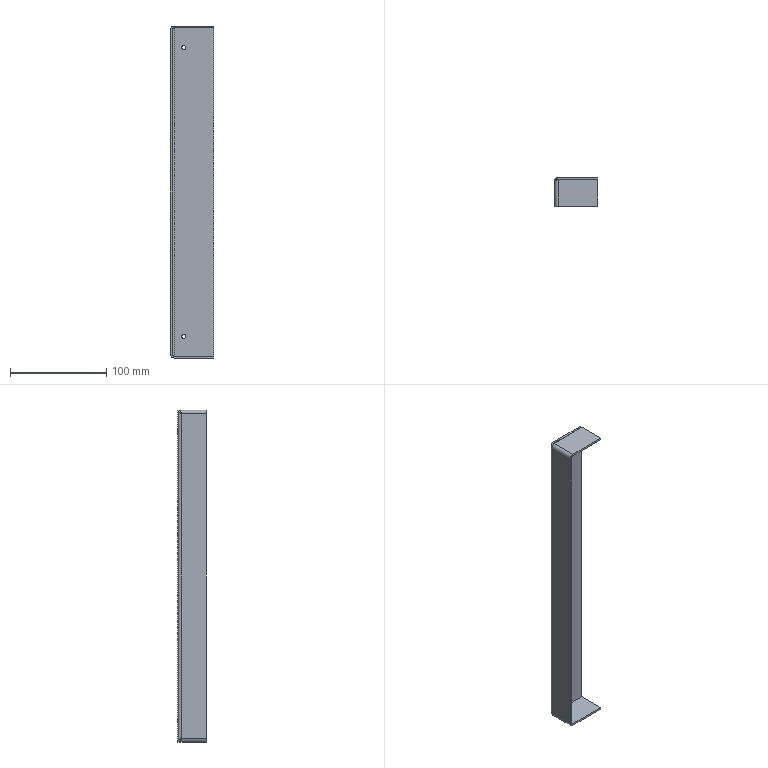Part | STEP file | SYL_0392D6J1SYL0380DJ1006-92088 | 1 solid | 34 faces | box 45 x 30 x 345 mm | volume 53987 mm3 | plane 20 | cylinder 10 | spline 4 | commonest cylinder face diameters 4.2 x4 4 x3 8 x3
STEP:
#1=CARTESIAN_POINT('',(-8.5,28.,-152.1));
#2=VERTEX_POINT('',#1);
#3=CARTESIAN_POINT('',(-8.5,30.,-152.1));
#4=VERTEX_POINT('',#3);
#5=CARTESIAN_POINT('',(-8.5,30.,-152.1));
#6=DIRECTION('',(0.,1.,0.));
#7=VECTOR('',#6,1000.);
#8=LINE('',#5,#7);
#9=EDGE_CURVE('',#2,#4,#8,.T.);
#10=ORIENTED_EDGE('',*,*,#9,.F.);
#11=CARTESIAN_POINT('',(-8.5,28.,-147.9));
#12=VERTEX_POINT('',#11);
#13=CARTESIAN_POINT('',(-8.5,28.,-150.));
#14=DIRECTION('',(0.,-1.,0.));
#15=DIRECTION('',(0.,0.,-1.));
#16=AXIS2_PLACEMENT_3D('',#13,#14,#15);
#17=CIRCLE('',#16,2.1);
#18=EDGE_CURVE('',#2,#12,#17,.T.);
#19=ORIENTED_EDGE('',*,*,#18,.T.);
#20=CARTESIAN_POINT('',(-8.5,30.,-147.9));
#21=VERTEX_POINT('',#20);
#22=CARTESIAN_POINT('',(-8.5,30.,-147.9));
#23=DIRECTION('',(0.,1.,0.));
#24=VECTOR('',#23,1000.);
#25=LINE('',#22,#24);
#26=EDGE_CURVE('',#12,#21,#25,.T.);
#27=ORIENTED_EDGE('',*,*,#26,.T.);
#28=CARTESIAN_POINT('',(-8.5,30.,-150.));
#29=DIRECTION('',(0.,-1.,0.));
#30=DIRECTION('',(0.,0.,-1.));
#31=AXIS2_PLACEMENT_3D('',#28,#29,#30);
#32=CIRCLE('',#31,2.1);
#33=EDGE_CURVE('',#4,#21,#32,.T.);
#34=ORIENTED_EDGE('',*,*,#33,.F.);
#35=EDGE_LOOP('',(#10,#19,#27,#34));
#36=FACE_OUTER_BOUND('',#35,.T.);
#37=CARTESIAN_POINT('',(-8.5,30.,-150.));
#38=DIRECTION('',(0.,1.,0.));
#39=DIRECTION('',(0.,0.,1.));
#40=AXIS2_PLACEMENT_3D('',#37,#38,#39);
#41=CYLINDRICAL_SURFACE('',#40,2.1);
#42=ADVANCED_FACE('',(#36),#41,.F.);
#43=CARTESIAN_POINT('',(-8.5,28.,147.9));
#44=VERTEX_POINT('',#43);
#45=CARTESIAN_POINT('',(-8.5,30.,147.9));
#46=VERTEX_POINT('',#45);
#47=CARTESIAN_POINT('',(-8.5,30.,147.9));
#48=DIRECTION('',(0.,1.,0.));
#49=VECTOR('',#48,1000.);
#50=LINE('',#47,#49);
#51=EDGE_CURVE('',#44,#46,#50,.T.);
#52=ORIENTED_EDGE('',*,*,#51,.F.);
#53=CARTESIAN_POINT('',(-8.5,28.,152.1));
#54=VERTEX_POINT('',#53);
#55=CARTESIAN_POINT('',(-8.5,28.,150.));
#56=DIRECTION('',(0.,-1.,0.));
#57=DIRECTION('',(0.,0.,-1.));
#58=AXIS2_PLACEMENT_3D('',#55,#56,#57);
#59=CIRCLE('',#58,2.1);
#60=EDGE_CURVE('',#44,#54,#59,.T.);
#61=ORIENTED_EDGE('',*,*,#60,.T.);
#62=CARTESIAN_POINT('',(-8.5,30.,152.1));
#63=VERTEX_POINT('',#62);
#64=CARTESIAN_POINT('',(-8.5,30.,152.1));
#65=DIRECTION('',(0.,1.,0.));
#66=VECTOR('',#65,1000.);
#67=LINE('',#64,#66);
#68=EDGE_CURVE('',#54,#63,#67,.T.);
#69=ORIENTED_EDGE('',*,*,#68,.T.);
#70=CARTESIAN_POINT('',(-8.5,30.,150.));
#71=DIRECTION('',(0.,-1.,0.));
#72=DIRECTION('',(0.,0.,-1.));
#73=AXIS2_PLACEMENT_3D('',#70,#71,#72);
#74=CIRCLE('',#73,2.1);
#75=EDGE_CURVE('',#46,#63,#74,.T.);
#76=ORIENTED_EDGE('',*,*,#75,.F.);
#77=EDGE_LOOP('',(#52,#61,#69,#76));
#78=FACE_OUTER_BOUND('',#77,.T.);
#79=CARTESIAN_POINT('',(-8.5,30.,150.));
#80=DIRECTION('',(0.,1.,0.));
#81=DIRECTION('',(0.,0.,1.));
#82=AXIS2_PLACEMENT_3D('',#79,#80,#81);
#83=CYLINDRICAL_SURFACE('',#82,2.1);
#84=ADVANCED_FACE('',(#78),#83,.F.);
#85=CARTESIAN_POINT('',(22.5,27.5,-170.5));
#86=VERTEX_POINT('',#85);
#87=CARTESIAN_POINT('',(22.5,27.5,-172.5));
#88=VERTEX_POINT('',#87);
#89=CARTESIAN_POINT('',(22.5,27.5,-172.5));
#90=DIRECTION('',(0.,0.,-1.));
#91=VECTOR('',#90,1000.);
#92=LINE('',#89,#91);
#93=EDGE_CURVE('',#86,#88,#92,.T.);
#94=ORIENTED_EDGE('',*,*,#93,.F.);
#95=CARTESIAN_POINT('',(22.5,0.,-170.5));
#96=VERTEX_POINT('',#95);
#97=CARTESIAN_POINT('',(22.5,26.,-170.5));
#98=DIRECTION('',(0.,1.,0.));
#99=VECTOR('',#98,1000.);
#100=LINE('',#97,#99);
#101=EDGE_CURVE('',#96,#86,#100,.T.);
#102=ORIENTED_EDGE('',*,*,#101,.F.);
#103=CARTESIAN_POINT('',(22.5,0.,-172.5));
#104=VERTEX_POINT('',#103);
#105=CARTESIAN_POINT('',(22.5,0.,-172.5));
#106=DIRECTION('',(0.,0.,-1.));
#107=VECTOR('',#106,1000.);
#108=LINE('',#105,#107);
#109=EDGE_CURVE('',#96,#104,#108,.T.);
#110=ORIENTED_EDGE('',*,*,#109,.T.);
#111=CARTESIAN_POINT('',(22.5,0.,-172.5));
#112=DIRECTION('',(0.,1.,0.));
#113=VECTOR('',#112,1000.);
#114=LINE('',#111,#113);
#115=EDGE_CURVE('',#104,#88,#114,.T.);
#116=ORIENTED_EDGE('',*,*,#115,.T.);
#117=EDGE_LOOP('',(#94,#102,#110,#116));
#118=FACE_OUTER_BOUND('',#117,.T.);
#119=CARTESIAN_POINT('',(22.5,0.,-172.5));
#120=DIRECTION('',(-1.,0.,0.));
#121=DIRECTION('',(0.,1.,0.));
#122=AXIS2_PLACEMENT_3D('',#119,#120,#121);
#123=PLANE('',#122);
#124=ADVANCED_FACE('',(#118),#123,.F.);
#125=ORIENTED_EDGE('',*,*,#109,.F.);
#126=CARTESIAN_POINT('',(-18.5,0.,-170.5));
#127=VERTEX_POINT('',#126);
#128=CARTESIAN_POINT('',(-22.5,0.,-170.5));
#129=DIRECTION('',(1.,0.,0.));
#130=VECTOR('',#129,1000.);
#131=LINE('',#128,#130);
#132=EDGE_CURVE('',#127,#96,#131,.T.);
#133=ORIENTED_EDGE('',*,*,#132,.F.);
#134=CARTESIAN_POINT('',(-18.5,0.,-172.5));
#135=VERTEX_POINT('',#134);
#136=CARTESIAN_POINT('',(-18.5,0.,-172.5));
#137=DIRECTION('',(0.,0.,-1.));
#138=VECTOR('',#137,1000.);
#139=LINE('',#136,#138);
#140=EDGE_CURVE('',#127,#135,#139,.T.);
#141=ORIENTED_EDGE('',*,*,#140,.T.);
#142=CARTESIAN_POINT('',(-18.5,0.,-172.5));
#143=DIRECTION('',(1.,0.,0.));
#144=VECTOR('',#143,1000.);
#145=LINE('',#142,#144);
#146=EDGE_CURVE('',#135,#104,#145,.T.);
#147=ORIENTED_EDGE('',*,*,#146,.T.);
#148=EDGE_LOOP('',(#125,#133,#141,#147));
#149=FACE_OUTER_BOUND('',#148,.T.);
#150=CARTESIAN_POINT('',(-18.5,0.,-172.5));
#151=DIRECTION('',(0.,1.,0.));
#152=DIRECTION('',(1.,0.,0.));
#153=AXIS2_PLACEMENT_3D('',#150,#151,#152);
#154=PLANE('',#153);
#155=ADVANCED_FACE('',(#149),#154,.F.);
#156=ORIENTED_EDGE('',*,*,#140,.F.);
#157=CARTESIAN_POINT('',(-20.5,0.,-168.5));
#158=VERTEX_POINT('',#157);
#159=CARTESIAN_POINT('',(-18.5,0.,-168.5));
#160=DIRECTION('',(0.,-1.,0.));
#161=DIRECTION('',(0.,0.,1.));
#162=AXIS2_PLACEMENT_3D('',#159,#160,#161);
#163=CIRCLE('',#162,2.);
#164=EDGE_CURVE('',#158,#127,#163,.T.);
#165=ORIENTED_EDGE('',*,*,#164,.F.);
#166=CARTESIAN_POINT('',(-22.5,0.,-168.5));
#167=VERTEX_POINT('',#166);
#168=CARTESIAN_POINT('',(-22.5,0.,-168.5));
#169=DIRECTION('',(-1.,0.,0.));
#170=VECTOR('',#169,1000.);
#171=LINE('',#168,#170);
#172=EDGE_CURVE('',#158,#167,#171,.T.);
#173=ORIENTED_EDGE('',*,*,#172,.T.);
#174=CARTESIAN_POINT('',(-18.5,0.,-168.5));
#175=DIRECTION('',(0.,-1.,0.));
#176=DIRECTION('',(-1.,0.,0.));
#177=AXIS2_PLACEMENT_3D('',#174,#175,#176);
#178=CIRCLE('',#177,4.);
#179=EDGE_CURVE('',#167,#135,#178,.T.);
#180=ORIENTED_EDGE('',*,*,#179,.T.);
#181=EDGE_LOOP('',(#156,#165,#173,#180));
#182=FACE_OUTER_BOUND('',#181,.T.);
#183=CARTESIAN_POINT('',(-18.5,0.,-168.5));
#184=DIRECTION('',(0.,1.,0.));
#185=DIRECTION('',(0.,0.,1.));
#186=AXIS2_PLACEMENT_3D('',#183,#184,#185);
#187=PLANE('',#186);
#188=ADVANCED_FACE('',(#182),#187,.F.);
#189=ORIENTED_EDGE('',*,*,#172,.F.);
#190=CARTESIAN_POINT('',(-20.5,0.,168.5));
#191=VERTEX_POINT('',#190);
#192=CARTESIAN_POINT('',(-20.5,0.,-172.5));
#193=DIRECTION('',(0.,0.,-1.));
#194=VECTOR('',#193,1000.);
#195=LINE('',#192,#194);
#196=EDGE_CURVE('',#191,#158,#195,.T.);
#197=ORIENTED_EDGE('',*,*,#196,.F.);
#198=CARTESIAN_POINT('',(-22.5,0.,168.5));
#199=VERTEX_POINT('',#198);
#200=CARTESIAN_POINT('',(-22.5,0.,168.5));
#201=DIRECTION('',(-1.,0.,0.));
#202=VECTOR('',#201,1000.);
#203=LINE('',#200,#202);
#204=EDGE_CURVE('',#191,#199,#203,.T.);
#205=ORIENTED_EDGE('',*,*,#204,.T.);
#206=CARTESIAN_POINT('',(-22.5,0.,168.5));
#207=DIRECTION('',(0.,0.,-1.));
#208=VECTOR('',#207,1000.);
#209=LINE('',#206,#208);
#210=EDGE_CURVE('',#199,#167,#209,.T.);
#211=ORIENTED_EDGE('',*,*,#210,.T.);
#212=EDGE_LOOP('',(#189,#197,#205,#211));
#213=FACE_OUTER_BOUND('',#212,.T.);
#214=CARTESIAN_POINT('',(-22.5,0.,168.5));
#215=DIRECTION('',(0.,1.,0.));
#216=DIRECTION('',(0.,0.,-1.));
#217=AXIS2_PLACEMENT_3D('',#214,#215,#216);
#218=PLANE('',#217);
#219=ADVANCED_FACE('',(#213),#218,.F.);
#220=ORIENTED_EDGE('',*,*,#204,.F.);
#221=CARTESIAN_POINT('',(-18.5,0.,170.5));
#222=VERTEX_POINT('',#221);
#223=CARTESIAN_POINT('',(-18.5,0.,168.5));
#224=DIRECTION('',(0.,-1.,0.));
#225=DIRECTION('',(0.,0.,-1.));
#226=AXIS2_PLACEMENT_3D('',#223,#224,#225);
#227=CIRCLE('',#226,2.);
#228=EDGE_CURVE('',#222,#191,#227,.T.);
#229=ORIENTED_EDGE('',*,*,#228,.F.);
#230=CARTESIAN_POINT('',(-18.5,0.,172.5));
#231=VERTEX_POINT('',#230);
#232=CARTESIAN_POINT('',(-18.5,0.,172.5));
#233=DIRECTION('',(0.,0.,1.));
#234=VECTOR('',#233,1000.);
#235=LINE('',#232,#234);
#236=EDGE_CURVE('',#222,#231,#235,.T.);
#237=ORIENTED_EDGE('',*,*,#236,.T.);
#238=CARTESIAN_POINT('',(-18.5,0.,168.5));
#239=DIRECTION('',(0.,-1.,0.));
#240=DIRECTION('',(0.,0.,1.));
#241=AXIS2_PLACEMENT_3D('',#238,#239,#240);
#242=CIRCLE('',#241,4.);
#243=EDGE_CURVE('',#231,#199,#242,.T.);
#244=ORIENTED_EDGE('',*,*,#243,.T.);
#245=EDGE_LOOP('',(#220,#229,#237,#244));
#246=FACE_OUTER_BOUND('',#245,.T.);
#247=CARTESIAN_POINT('',(-18.5,0.,168.5));
#248=DIRECTION('',(0.,1.,0.));
#249=DIRECTION('',(0.,0.,1.));
#250=AXIS2_PLACEMENT_3D('',#247,#248,#249);
#251=PLANE('',#250);
#252=ADVANCED_FACE('',(#246),#251,.F.);
#253=ORIENTED_EDGE('',*,*,#236,.F.);
#254=CARTESIAN_POINT('',(22.5,0.,170.5));
#255=VERTEX_POINT('',#254);
#256=CARTESIAN_POINT('',(-22.5,0.,170.5));
#257=DIRECTION('',(-1.,0.,0.));
#258=VECTOR('',#257,1000.);
#259=LINE('',#256,#258);
#260=EDGE_CURVE('',#255,#222,#259,.T.);
#261=ORIENTED_EDGE('',*,*,#260,.F.);
#262=CARTESIAN_POINT('',(22.5,0.,172.5));
#263=VERTEX_POINT('',#262);
#264=CARTESIAN_POINT('',(22.5,0.,172.5));
#265=DIRECTION('',(0.,0.,1.));
#266=VECTOR('',#265,1000.);
#267=LINE('',#264,#266);
#268=EDGE_CURVE('',#255,#263,#267,.T.);
#269=ORIENTED_EDGE('',*,*,#268,.T.);
#270=CARTESIAN_POINT('',(22.5,0.,172.5));
#271=DIRECTION('',(-1.,0.,0.));
#272=VECTOR('',#271,1000.);
#273=LINE('',#270,#272);
#274=EDGE_CURVE('',#263,#231,#273,.T.);
#275=ORIENTED_EDGE('',*,*,#274,.T.);
#276=EDGE_LOOP('',(#253,#261,#269,#275));
#277=FACE_OUTER_BOUND('',#276,.T.);
#278=CARTESIAN_POINT('',(22.5,0.,172.5));
#279=DIRECTION('',(0.,1.,0.));
#280=DIRECTION('',(-1.,0.,0.));
#281=AXIS2_PLACEMENT_3D('',#278,#279,#280);
#282=PLANE('',#281);
#283=ADVANCED_FACE('',(#277),#282,.F.);
#284=ORIENTED_EDGE('',*,*,#268,.F.);
#285=CARTESIAN_POINT('',(22.5,27.5,170.5));
#286=VERTEX_POINT('',#285);
#287=CARTESIAN_POINT('',(22.5,0.,170.5));
#288=DIRECTION('',(0.,-1.,0.));
#289=VECTOR('',#288,1000.);
#290=LINE('',#287,#289);
#291=EDGE_CURVE('',#286,#255,#290,.T.);
#292=ORIENTED_EDGE('',*,*,#291,.F.);
#293=CARTESIAN_POINT('',(22.5,27.5,172.5));
#294=VERTEX_POINT('',#293);
#295=CARTESIAN_POINT('',(22.5,27.5,172.5));
#296=DIRECTION('',(0.,0.,1.));
#297=VECTOR('',#296,1000.);
#298=LINE('',#295,#297);
#299=EDGE_CURVE('',#286,#294,#298,.T.);
#300=ORIENTED_EDGE('',*,*,#299,.T.);
#301=CARTESIAN_POINT('',(22.5,27.5,172.5));
#302=DIRECTION('',(0.,-1.,0.));
#303=VECTOR('',#302,1000.);
#304=LINE('',#301,#303);
#305=EDGE_CURVE('',#294,#263,#304,.T.);
#306=ORIENTED_EDGE('',*,*,#305,.T.);
#307=EDGE_LOOP('',(#284,#292,#300,#306));
#308=FACE_OUTER_BOUND('',#307,.T.);
#309=CARTESIAN_POINT('',(22.5,27.5,172.5));
#310=DIRECTION('',(-1.,0.,0.));
#311=DIRECTION('',(0.,-1.,0.));
#312=AXIS2_PLACEMENT_3D('',#309,#310,#311);
#313=PLANE('',#312);
#314=ADVANCED_FACE('',(#308),#313,.F.);
#315=ORIENTED_EDGE('',*,*,#299,.F.);
#316=CARTESIAN_POINT('',(-18.5,27.5,170.5));
#317=VERTEX_POINT('',#316);
#318=CARTESIAN_POINT('',(-22.5,27.5,170.5));
#319=DIRECTION('',(1.,0.,0.));
#320=VECTOR('',#319,1000.);
#321=LINE('',#318,#320);
#322=EDGE_CURVE('',#317,#286,#321,.T.);
#323=ORIENTED_EDGE('',*,*,#322,.F.);
#324=CARTESIAN_POINT('',(-18.5,27.5,172.5));
#325=VERTEX_POINT('',#324);
#326=CARTESIAN_POINT('',(-18.5,27.5,170.5));
#327=CARTESIAN_POINT('',(-18.5,27.5,171.167));
#328=CARTESIAN_POINT('',(-18.5,27.5,171.833));
#329=CARTESIAN_POINT('',(-18.5,27.5,172.5));
#330=B_SPLINE_CURVE_WITH_KNOTS('',3,(#326,#327,#328,#329),.UNSPECIFIED.,.F.,.F.,(4,4),(0.,1.),.UNSPECIFIED.);
#331=EDGE_CURVE('',#317,#325,#330,.T.);
#332=ORIENTED_EDGE('',*,*,#331,.T.);
#333=CARTESIAN_POINT('',(-18.5,27.5,172.5));
#334=DIRECTION('',(1.,0.,0.));
#335=VECTOR('',#334,1000.);
#336=LINE('',#333,#335);
#337=EDGE_CURVE('',#325,#294,#336,.T.);
#338=ORIENTED_EDGE('',*,*,#337,.T.);
#339=EDGE_LOOP('',(#315,#323,#332,#338));
#340=FACE_OUTER_BOUND('',#339,.T.);
#341=CARTESIAN_POINT('',(-18.5,27.5,172.5));
#342=DIRECTION('',(0.,-1.,0.));
#343=DIRECTION('',(1.,0.,0.));
#344=AXIS2_PLACEMENT_3D('',#341,#342,#343);
#345=PLANE('',#344);
#346=ADVANCED_FACE('',(#340),#345,.F.);
#347=ORIENTED_EDGE('',*,*,#331,.F.);
#348=CARTESIAN_POINT('',(-20.5,26.,168.5));
#349=VERTEX_POINT('',#348);
#350=CARTESIAN_POINT('',(-18.5,27.5,170.5));
#351=CARTESIAN_POINT('',(-18.762,27.375,170.5));
#352=CARTESIAN_POINT('',(-19.023,27.25,170.448));
#353=CARTESIAN_POINT('',(-19.507,27.,170.248));
#354=CARTESIAN_POINT('',(-19.729,26.875,170.099));
#355=CARTESIAN_POINT('',(-20.099,26.625,169.729));
#356=CARTESIAN_POINT('',(-20.248,26.5,169.507));
#357=CARTESIAN_POINT('',(-20.448,26.25,169.023));
#358=CARTESIAN_POINT('',(-20.5,26.125,168.762));
#359=CARTESIAN_POINT('',(-20.5,26.,168.5));
#360=B_SPLINE_CURVE_WITH_KNOTS('',3,(#350,#351,#352,#353,#354,#355,#356,#357,#358,#359),.UNSPECIFIED.,.F.,.F.,(4,2,2,2,4),(0.,0.25,0.5,0.75,1.),.UNSPECIFIED.);
#361=EDGE_CURVE('',#317,#349,#360,.T.);
#362=ORIENTED_EDGE('',*,*,#361,.T.);
#363=CARTESIAN_POINT('',(-22.5,26.,168.5));
#364=VERTEX_POINT('',#363);
#365=CARTESIAN_POINT('',(-20.5,26.,168.5));
#366=CARTESIAN_POINT('',(-22.5,26.,168.5));
#367=B_SPLINE_CURVE_WITH_KNOTS('',1,(#365,#366),.UNSPECIFIED.,.F.,.F.,(2,2),(0.,1.),.UNSPECIFIED.);
#368=EDGE_CURVE('',#349,#364,#367,.T.);
#369=ORIENTED_EDGE('',*,*,#368,.T.);
#370=CARTESIAN_POINT('',(-18.5,27.5,172.5));
#371=CARTESIAN_POINT('',(-19.024,27.375,172.5));
#372=CARTESIAN_POINT('',(-19.547,27.25,172.396));
#373=CARTESIAN_POINT('',(-20.514,27.,171.995));
#374=CARTESIAN_POINT('',(-20.958,26.875,171.699));
#375=CARTESIAN_POINT('',(-21.699,26.625,170.958));
#376=CARTESIAN_POINT('',(-21.995,26.5,170.514));
#377=CARTESIAN_POINT('',(-22.396,26.25,169.547));
#378=CARTESIAN_POINT('',(-22.5,26.125,169.024));
#379=CARTESIAN_POINT('',(-22.5,26.,168.5));
#380=B_SPLINE_CURVE_WITH_KNOTS('',3,(#370,#371,#372,#373,#374,#375,#376,#377,#378,#379),.UNSPECIFIED.,.F.,.F.,(4,2,2,2,4),(0.,0.25,0.5,0.75,1.),.UNSPECIFIED.);
#381=EDGE_CURVE('',#325,#364,#380,.T.);
#382=ORIENTED_EDGE('',*,*,#381,.F.);
#383=EDGE_LOOP('',(#347,#362,#369,#382));
#384=FACE_OUTER_BOUND('',#383,.T.);
#385=CARTESIAN_POINT('',(-18.5,27.5,172.5));
#386=CARTESIAN_POINT('',(-19.024,27.375,172.5));
#387=CARTESIAN_POINT('',(-19.547,27.25,172.396));
#388=CARTESIAN_POINT('',(-20.514,27.,171.995));
#389=CARTESIAN_POINT('',(-20.958,26.875,171.699));
#390=CARTESIAN_POINT('',(-21.699,26.625,170.958));
#391=CARTESIAN_POINT('',(-21.995,26.5,170.514));
#392=CARTESIAN_POINT('',(-22.396,26.25,169.547));
#393=CARTESIAN_POINT('',(-22.5,26.125,169.024));
#394=CARTESIAN_POINT('',(-22.5,26.,168.5));
#395=CARTESIAN_POINT('',(-18.5,27.5,170.5));
#396=CARTESIAN_POINT('',(-18.762,27.375,170.5));
#397=CARTESIAN_POINT('',(-19.023,27.25,170.448));
#398=CARTESIAN_POINT('',(-19.507,27.,170.248));
#399=CARTESIAN_POINT('',(-19.729,26.875,170.099));
#400=CARTESIAN_POINT('',(-20.099,26.625,169.729));
#401=CARTESIAN_POINT('',(-20.248,26.5,169.507));
#402=CARTESIAN_POINT('',(-20.448,26.25,169.023));
#403=CARTESIAN_POINT('',(-20.5,26.125,168.762));
#404=CARTESIAN_POINT('',(-20.5,26.,168.5));
#405=B_SPLINE_SURFACE_WITH_KNOTS('',1,3,((#385,#386,#387,#388,#389,#390,#391,#392,#393,#394),(#395,#396,#397,#398,#399,#400,#401,#402,#403,#404)),.UNSPECIFIED.,.F.,.F.,.F.,(2,2),(4,2,2,2,4),(0.,1.),(0.,0.25,0.5,0.75,1.),.UNSPECIFIED.);
#406=ADVANCED_FACE('',(#384),#405,.T.);
#407=ORIENTED_EDGE('',*,*,#368,.F.);
#408=CARTESIAN_POINT('',(-18.5,28.,172.5));
#409=VERTEX_POINT('',#408);
#410=CARTESIAN_POINT('',(-20.5,26.,168.5));
#411=CARTESIAN_POINT('',(-20.5,26.262,168.833));
#412=CARTESIAN_POINT('',(-20.448,26.523,169.167));
#413=CARTESIAN_POINT('',(-20.248,27.007,169.833));
#414=CARTESIAN_POINT('',(-20.099,27.229,170.167));
#415=CARTESIAN_POINT('',(-19.729,27.599,170.833));
#416=CARTESIAN_POINT('',(-19.507,27.748,171.167));
#417=CARTESIAN_POINT('',(-19.023,27.948,171.833));
#418=CARTESIAN_POINT('',(-18.762,28.,172.167));
#419=CARTESIAN_POINT('',(-18.5,28.,172.5));
#420=B_SPLINE_CURVE_WITH_KNOTS('',3,(#410,#411,#412,#413,#414,#415,#416,#417,#418,#419),.UNSPECIFIED.,.F.,.F.,(4,2,2,2,4),(0.,0.25,0.5,0.75,1.),.UNSPECIFIED.);
#421=EDGE_CURVE('',#349,#409,#420,.T.);
#422=ORIENTED_EDGE('',*,*,#421,.T.);
#423=CARTESIAN_POINT('',(-18.5,30.,172.5));
#424=VERTEX_POINT('',#423);
#425=CARTESIAN_POINT('',(-18.5,28.,172.5));
#426=CARTESIAN_POINT('',(-18.5,30.,172.5));
#427=B_SPLINE_CURVE_WITH_KNOTS('',1,(#425,#426),.UNSPECIFIED.,.F.,.F.,(2,2),(0.,1.),.UNSPECIFIED.);
#428=EDGE_CURVE('',#409,#424,#427,.T.);
#429=ORIENTED_EDGE('',*,*,#428,.T.);
#430=CARTESIAN_POINT('',(-22.5,26.,168.5));
#431=CARTESIAN_POINT('',(-22.5,26.524,168.833));
#432=CARTESIAN_POINT('',(-22.396,27.047,169.167));
#433=CARTESIAN_POINT('',(-21.995,28.014,169.833));
#434=CARTESIAN_POINT('',(-21.699,28.458,170.167));
#435=CARTESIAN_POINT('',(-20.958,29.199,170.833));
#436=CARTESIAN_POINT('',(-20.514,29.495,171.167));
#437=CARTESIAN_POINT('',(-19.547,29.896,171.833));
#438=CARTESIAN_POINT('',(-19.024,30.,172.167));
#439=CARTESIAN_POINT('',(-18.5,30.,172.5));
#440=B_SPLINE_CURVE_WITH_KNOTS('',3,(#430,#431,#432,#433,#434,#435,#436,#437,#438,#439),.UNSPECIFIED.,.F.,.F.,(4,2,2,2,4),(0.,0.25,0.5,0.75,1.),.UNSPECIFIED.);
#441=EDGE_CURVE('',#364,#424,#440,.T.);
#442=ORIENTED_EDGE('',*,*,#441,.F.);
#443=EDGE_LOOP('',(#407,#422,#429,#442));
#444=FACE_OUTER_BOUND('',#443,.T.);
#445=CARTESIAN_POINT('',(-22.5,26.,168.5));
#446=CARTESIAN_POINT('',(-22.5,26.524,168.833));
#447=CARTESIAN_POINT('',(-22.396,27.047,169.167));
#448=CARTESIAN_POINT('',(-21.995,28.014,169.833));
#449=CARTESIAN_POINT('',(-21.699,28.458,170.167));
#450=CARTESIAN_POINT('',(-20.958,29.199,170.833));
#451=CARTESIAN_POINT('',(-20.514,29.495,171.167));
#452=CARTESIAN_POINT('',(-19.547,29.896,171.833));
#453=CARTESIAN_POINT('',(-19.024,30.,172.167));
#454=CARTESIAN_POINT('',(-18.5,30.,172.5));
#455=CARTESIAN_POINT('',(-20.5,26.,168.5));
#456=CARTESIAN_POINT('',(-20.5,26.262,168.833));
#457=CARTESIAN_POINT('',(-20.448,26.523,169.167));
#458=CARTESIAN_POINT('',(-20.248,27.007,169.833));
#459=CARTESIAN_POINT('',(-20.099,27.229,170.167));
#460=CARTESIAN_POINT('',(-19.729,27.599,170.833));
#461=CARTESIAN_POINT('',(-19.507,27.748,171.167));
#462=CARTESIAN_POINT('',(-19.023,27.948,171.833));
#463=CARTESIAN_POINT('',(-18.762,28.,172.167));
#464=CARTESIAN_POINT('',(-18.5,28.,172.5));
#465=B_SPLINE_SURFACE_WITH_KNOTS('',1,3,((#445,#446,#447,#448,#449,#450,#451,#452,#453,#454),(#455,#456,#457,#458,#459,#460,#461,#462,#463,#464)),.UNSPECIFIED.,.F.,.F.,.F.,(2,2),(4,2,2,2,4),(0.,1.),(0.,0.25,0.5,0.75,1.),.UNSPECIFIED.);
#466=ADVANCED_FACE('',(#444),#465,.T.);
#467=ORIENTED_EDGE('',*,*,#428,.F.);
#468=CARTESIAN_POINT('',(22.5,28.,172.5));
#469=VERTEX_POINT('',#468);
#470=CARTESIAN_POINT('',(22.5,28.,172.5));
#471=DIRECTION('',(-1.,0.,0.));
#472=VECTOR('',#471,1000.);
#473=LINE('',#470,#472);
#474=EDGE_CURVE('',#469,#409,#473,.T.);
#475=ORIENTED_EDGE('',*,*,#474,.F.);
#476=CARTESIAN_POINT('',(22.5,30.,172.5));
#477=VERTEX_POINT('',#476);
#478=CARTESIAN_POINT('',(22.5,30.,172.5));
#479=DIRECTION('',(0.,1.,0.));
#480=VECTOR('',#479,1000.);
#481=LINE('',#478,#480);
#482=EDGE_CURVE('',#469,#477,#481,.T.);
#483=ORIENTED_EDGE('',*,*,#482,.T.);
#484=CARTESIAN_POINT('',(22.5,30.,172.5));
#485=DIRECTION('',(-1.,0.,0.));
#486=VECTOR('',#485,1000.);
#487=LINE('',#484,#486);
#488=EDGE_CURVE('',#477,#424,#487,.T.);
#489=ORIENTED_EDGE('',*,*,#488,.T.);
#490=EDGE_LOOP('',(#467,#475,#483,#489));
#491=FACE_OUTER_BOUND('',#490,.T.);
#492=CARTESIAN_POINT('',(22.5,30.,172.5));
#493=DIRECTION('',(0.,0.,-1.));
#494=DIRECTION('',(-1.,0.,0.));
#495=AXIS2_PLACEMENT_3D('',#492,#493,#494);
#496=PLANE('',#495);
#497=ADVANCED_FACE('',(#491),#496,.F.);
#498=ORIENTED_EDGE('',*,*,#482,.F.);
#499=CARTESIAN_POINT('',(22.5,28.,-172.5));
#500=VERTEX_POINT('',#499);
#501=CARTESIAN_POINT('',(22.5,28.,-172.5));
#502=DIRECTION('',(0.,0.,1.));
#503=VECTOR('',#502,1000.);
#504=LINE('',#501,#503);
#505=EDGE_CURVE('',#500,#469,#504,.T.);
#506=ORIENTED_EDGE('',*,*,#505,.F.);
#507=CARTESIAN_POINT('',(22.5,30.,-172.5));
#508=VERTEX_POINT('',#507);
#509=CARTESIAN_POINT('',(22.5,30.,-172.5));
#510=DIRECTION('',(0.,1.,0.));
#511=VECTOR('',#510,1000.);
#512=LINE('',#509,#511);
#513=EDGE_CURVE('',#500,#508,#512,.T.);
#514=ORIENTED_EDGE('',*,*,#513,.T.);
#515=CARTESIAN_POINT('',(22.5,30.,-172.5));
#516=DIRECTION('',(0.,0.,1.));
#517=VECTOR('',#516,1000.);
#518=LINE('',#515,#517);
#519=EDGE_CURVE('',#508,#477,#518,.T.);
#520=ORIENTED_EDGE('',*,*,#519,.T.);
#521=EDGE_LOOP('',(#498,#506,#514,#520));
#522=FACE_OUTER_BOUND('',#521,.T.);
#523=CARTESIAN_POINT('',(22.5,30.,-172.5));
#524=DIRECTION('',(-1.,0.,0.));
#525=DIRECTION('',(0.,0.,1.));
#526=AXIS2_PLACEMENT_3D('',#523,#524,#525);
#527=PLANE('',#526);
#528=ADVANCED_FACE('',(#522),#527,.F.);
#529=ORIENTED_EDGE('',*,*,#513,.F.);
#530=CARTESIAN_POINT('',(-18.5,28.,-172.5));
#531=VERTEX_POINT('',#530);
#532=CARTESIAN_POINT('',(22.5,28.,-172.5));
#533=DIRECTION('',(1.,0.,0.));
#534=VECTOR('',#533,1000.);
#535=LINE('',#532,#534);
#536=EDGE_CURVE('',#531,#500,#535,.T.);
#537=ORIENTED_EDGE('',*,*,#536,.F.);
#538=CARTESIAN_POINT('',(-18.5,30.,-172.5));
#539=VERTEX_POINT('',#538);
#540=CARTESIAN_POINT('',(-18.5,28.,-172.5));
#541=CARTESIAN_POINT('',(-18.5,28.667,-172.5));
#542=CARTESIAN_POINT('',(-18.5,29.333,-172.5));
#543=CARTESIAN_POINT('',(-18.5,30.,-172.5));
#544=B_SPLINE_CURVE_WITH_KNOTS('',3,(#540,#541,#542,#543),.UNSPECIFIED.,.F.,.F.,(4,4),(0.,1.),.UNSPECIFIED.);
#545=EDGE_CURVE('',#531,#539,#544,.T.);
#546=ORIENTED_EDGE('',*,*,#545,.T.);
#547=CARTESIAN_POINT('',(-18.5,30.,-172.5));
#548=DIRECTION('',(1.,0.,0.));
#549=VECTOR('',#548,1000.);
#550=LINE('',#547,#549);
#551=EDGE_CURVE('',#539,#508,#550,.T.);
#552=ORIENTED_EDGE('',*,*,#551,.T.);
#553=EDGE_LOOP('',(#529,#537,#546,#552));
#554=FACE_OUTER_BOUND('',#553,.T.);
#555=CARTESIAN_POINT('',(-18.5,30.,-172.5));
#556=DIRECTION('',(0.,0.,1.));
#557=DIRECTION('',(1.,0.,0.));
#558=AXIS2_PLACEMENT_3D('',#555,#556,#557);
#559=PLANE('',#558);
#560=ADVANCED_FACE('',(#554),#559,.F.);
#561=ORIENTED_EDGE('',*,*,#545,.F.);
#562=CARTESIAN_POINT('',(-20.5,26.,-168.5));
#563=VERTEX_POINT('',#562);
#564=CARTESIAN_POINT('',(-18.5,28.,-172.5));
#565=CARTESIAN_POINT('',(-18.762,28.,-172.167));
#566=CARTESIAN_POINT('',(-19.023,27.948,-171.833));
#567=CARTESIAN_POINT('',(-19.507,27.748,-171.167));
#568=CARTESIAN_POINT('',(-19.729,27.599,-170.833));
#569=CARTESIAN_POINT('',(-20.099,27.229,-170.167));
#570=CARTESIAN_POINT('',(-20.248,27.007,-169.833));
#571=CARTESIAN_POINT('',(-20.448,26.523,-169.167));
#572=CARTESIAN_POINT('',(-20.5,26.262,-168.833));
#573=CARTESIAN_POINT('',(-20.5,26.,-168.5));
#574=B_SPLINE_CURVE_WITH_KNOTS('',3,(#564,#565,#566,#567,#568,#569,#570,#571,#572,#573),.UNSPECIFIED.,.F.,.F.,(4,2,2,2,4),(0.,0.25,0.5,0.75,1.),.UNSPECIFIED.);
#575=EDGE_CURVE('',#531,#563,#574,.T.);
#576=ORIENTED_EDGE('',*,*,#575,.T.);
#577=CARTESIAN_POINT('',(-22.5,26.,-168.5));
#578=VERTEX_POINT('',#577);
#579=CARTESIAN_POINT('',(-20.5,26.,-168.5));
#580=CARTESIAN_POINT('',(-22.5,26.,-168.5));
#581=B_SPLINE_CURVE_WITH_KNOTS('',1,(#579,#580),.UNSPECIFIED.,.F.,.F.,(2,2),(0.,1.),.UNSPECIFIED.);
#582=EDGE_CURVE('',#563,#578,#581,.T.);
#583=ORIENTED_EDGE('',*,*,#582,.T.);
#584=CARTESIAN_POINT('',(-18.5,30.,-172.5));
#585=CARTESIAN_POINT('',(-19.024,30.,-172.167));
#586=CARTESIAN_POINT('',(-19.547,29.896,-171.833));
#587=CARTESIAN_POINT('',(-20.514,29.495,-171.167));
#588=CARTESIAN_POINT('',(-20.958,29.199,-170.833));
#589=CARTESIAN_POINT('',(-21.699,28.458,-170.167));
#590=CARTESIAN_POINT('',(-21.995,28.014,-169.833));
#591=CARTESIAN_POINT('',(-22.396,27.047,-169.167));
#592=CARTESIAN_POINT('',(-22.5,26.524,-168.833));
#593=CARTESIAN_POINT('',(-22.5,26.,-168.5));
#594=B_SPLINE_CURVE_WITH_KNOTS('',3,(#584,#585,#586,#587,#588,#589,#590,#591,#592,#593),.UNSPECIFIED.,.F.,.F.,(4,2,2,2,4),(0.,0.25,0.5,0.75,1.),.UNSPECIFIED.);
#595=EDGE_CURVE('',#539,#578,#594,.T.);
#596=ORIENTED_EDGE('',*,*,#595,.F.);
#597=EDGE_LOOP('',(#561,#576,#583,#596));
#598=FACE_OUTER_BOUND('',#597,.T.);
#599=CARTESIAN_POINT('',(-18.5,30.,-172.5));
#600=CARTESIAN_POINT('',(-19.024,30.,-172.167));
#601=CARTESIAN_POINT('',(-19.547,29.896,-171.833));
#602=CARTESIAN_POINT('',(-20.514,29.495,-171.167));
#603=CARTESIAN_POINT('',(-20.958,29.199,-170.833));
#604=CARTESIAN_POINT('',(-21.699,28.458,-170.167));
#605=CARTESIAN_POINT('',(-21.995,28.014,-169.833));
#606=CARTESIAN_POINT('',(-22.396,27.047,-169.167));
#607=CARTESIAN_POINT('',(-22.5,26.524,-168.833));
#608=CARTESIAN_POINT('',(-22.5,26.,-168.5));
#609=CARTESIAN_POINT('',(-18.5,28.,-172.5));
#610=CARTESIAN_POINT('',(-18.762,28.,-172.167));
#611=CARTESIAN_POINT('',(-19.023,27.948,-171.833));
#612=CARTESIAN_POINT('',(-19.507,27.748,-171.167));
#613=CARTESIAN_POINT('',(-19.729,27.599,-170.833));
#614=CARTESIAN_POINT('',(-20.099,27.229,-170.167));
#615=CARTESIAN_POINT('',(-20.248,27.007,-169.833));
#616=CARTESIAN_POINT('',(-20.448,26.523,-169.167));
#617=CARTESIAN_POINT('',(-20.5,26.262,-168.833));
#618=CARTESIAN_POINT('',(-20.5,26.,-168.5));
#619=B_SPLINE_SURFACE_WITH_KNOTS('',1,3,((#599,#600,#601,#602,#603,#604,#605,#606,#607,#608),(#609,#610,#611,#612,#613,#614,#615,#616,#617,#618)),.UNSPECIFIED.,.F.,.F.,.F.,(2,2),(4,2,2,2,4),(0.,1.),(0.,0.25,0.5,0.75,1.),.UNSPECIFIED.);
#620=ADVANCED_FACE('',(#598),#619,.T.);
#621=ORIENTED_EDGE('',*,*,#582,.F.);
#622=CARTESIAN_POINT('',(-18.5,27.5,-170.5));
#623=VERTEX_POINT('',#622);
#624=CARTESIAN_POINT('',(-20.5,26.,-168.5));
#625=CARTESIAN_POINT('',(-20.5,26.125,-168.762));
#626=CARTESIAN_POINT('',(-20.448,26.25,-169.023));
#627=CARTESIAN_POINT('',(-20.248,26.5,-169.507));
#628=CARTESIAN_POINT('',(-20.099,26.625,-169.729));
#629=CARTESIAN_POINT('',(-19.729,26.875,-170.099));
#630=CARTESIAN_POINT('',(-19.507,27.,-170.248));
#631=CARTESIAN_POINT('',(-19.023,27.25,-170.448));
#632=CARTESIAN_POINT('',(-18.762,27.375,-170.5));
#633=CARTESIAN_POINT('',(-18.5,27.5,-170.5));
#634=B_SPLINE_CURVE_WITH_KNOTS('',3,(#624,#625,#626,#627,#628,#629,#630,#631,#632,#633),.UNSPECIFIED.,.F.,.F.,(4,2,2,2,4),(0.,0.25,0.5,0.75,1.),.UNSPECIFIED.);
#635=EDGE_CURVE('',#563,#623,#634,.T.);
#636=ORIENTED_EDGE('',*,*,#635,.T.);
#637=CARTESIAN_POINT('',(-18.5,27.5,-172.5));
#638=VERTEX_POINT('',#637);
#639=CARTESIAN_POINT('',(-18.5,27.5,-170.5));
#640=CARTESIAN_POINT('',(-18.5,27.5,-172.5));
#641=B_SPLINE_CURVE_WITH_KNOTS('',1,(#639,#640),.UNSPECIFIED.,.F.,.F.,(2,2),(0.,1.),.UNSPECIFIED.);
#642=EDGE_CURVE('',#623,#638,#641,.T.);
#643=ORIENTED_EDGE('',*,*,#642,.T.);
#644=CARTESIAN_POINT('',(-22.5,26.,-168.5));
#645=CARTESIAN_POINT('',(-22.5,26.125,-169.024));
#646=CARTESIAN_POINT('',(-22.396,26.25,-169.547));
#647=CARTESIAN_POINT('',(-21.995,26.5,-170.514));
#648=CARTESIAN_POINT('',(-21.699,26.625,-170.958));
#649=CARTESIAN_POINT('',(-20.958,26.875,-171.699));
#650=CARTESIAN_POINT('',(-20.514,27.,-171.995));
#651=CARTESIAN_POINT('',(-19.547,27.25,-172.396));
#652=CARTESIAN_POINT('',(-19.024,27.375,-172.5));
#653=CARTESIAN_POINT('',(-18.5,27.5,-172.5));
#654=B_SPLINE_CURVE_WITH_KNOTS('',3,(#644,#645,#646,#647,#648,#649,#650,#651,#652,#653),.UNSPECIFIED.,.F.,.F.,(4,2,2,2,4),(0.,0.25,0.5,0.75,1.),.UNSPECIFIED.);
#655=EDGE_CURVE('',#578,#638,#654,.T.);
#656=ORIENTED_EDGE('',*,*,#655,.F.);
#657=EDGE_LOOP('',(#621,#636,#643,#656));
#658=FACE_OUTER_BOUND('',#657,.T.);
#659=CARTESIAN_POINT('',(-22.5,26.,-168.5));
#660=CARTESIAN_POINT('',(-22.5,26.125,-169.024));
#661=CARTESIAN_POINT('',(-22.396,26.25,-169.547));
#662=CARTESIAN_POINT('',(-21.995,26.5,-170.514));
#663=CARTESIAN_POINT('',(-21.699,26.625,-170.958));
#664=CARTESIAN_POINT('',(-20.958,26.875,-171.699));
#665=CARTESIAN_POINT('',(-20.514,27.,-171.995));
#666=CARTESIAN_POINT('',(-19.547,27.25,-172.396));
#667=CARTESIAN_POINT('',(-19.024,27.375,-172.5));
#668=CARTESIAN_POINT('',(-18.5,27.5,-172.5));
#669=CARTESIAN_POINT('',(-20.5,26.,-168.5));
#670=CARTESIAN_POINT('',(-20.5,26.125,-168.762));
#671=CARTESIAN_POINT('',(-20.448,26.25,-169.023));
#672=CARTESIAN_POINT('',(-20.248,26.5,-169.507));
#673=CARTESIAN_POINT('',(-20.099,26.625,-169.729));
#674=CARTESIAN_POINT('',(-19.729,26.875,-170.099));
#675=CARTESIAN_POINT('',(-19.507,27.,-170.248));
#676=CARTESIAN_POINT('',(-19.023,27.25,-170.448));
#677=CARTESIAN_POINT('',(-18.762,27.375,-170.5));
#678=CARTESIAN_POINT('',(-18.5,27.5,-170.5));
#679=B_SPLINE_SURFACE_WITH_KNOTS('',1,3,((#659,#660,#661,#662,#663,#664,#665,#666,#667,#668),(#669,#670,#671,#672,#673,#674,#675,#676,#677,#678)),.UNSPECIFIED.,.F.,.F.,.F.,(2,2),(4,2,2,2,4),(0.,1.),(0.,0.25,0.5,0.75,1.),.UNSPECIFIED.);
#680=ADVANCED_FACE('',(#658),#679,.T.);
#681=CARTESIAN_POINT('',(-8.5,28.,150.));
#682=DIRECTION('',(0.,-1.,0.));
#683=DIRECTION('',(0.,0.,-1.));
#684=AXIS2_PLACEMENT_3D('',#681,#682,#683);
#685=CIRCLE('',#684,2.1);
#686=EDGE_CURVE('',#54,#44,#685,.T.);
#687=ORIENTED_EDGE('',*,*,#686,.T.);
#688=ORIENTED_EDGE('',*,*,#51,.T.);
#689=CARTESIAN_POINT('',(-8.5,30.,150.));
#690=DIRECTION('',(0.,-1.,0.));
#691=DIRECTION('',(0.,0.,1.));
#692=AXIS2_PLACEMENT_3D('',#689,#690,#691);
#693=CIRCLE('',#692,2.1);
#694=EDGE_CURVE('',#63,#46,#693,.T.);
#695=ORIENTED_EDGE('',*,*,#694,.F.);
#696=ORIENTED_EDGE('',*,*,#68,.F.);
#697=EDGE_LOOP('',(#687,#688,#695,#696));
#698=FACE_OUTER_BOUND('',#697,.T.);
#699=CARTESIAN_POINT('',(-8.5,30.,150.));
#700=DIRECTION('',(0.,1.,0.));
#701=DIRECTION('',(0.,0.,1.));
#702=AXIS2_PLACEMENT_3D('',#699,#700,#701);
#703=CYLINDRICAL_SURFACE('',#702,2.1);
#704=ADVANCED_FACE('',(#698),#703,.F.);
#705=CARTESIAN_POINT('',(-8.5,28.,-150.));
#706=DIRECTION('',(0.,-1.,0.));
#707=DIRECTION('',(0.,0.,-1.));
#708=AXIS2_PLACEMENT_3D('',#705,#706,#707);
#709=CIRCLE('',#708,2.1);
#710=EDGE_CURVE('',#12,#2,#709,.T.);
#711=ORIENTED_EDGE('',*,*,#710,.T.);
#712=ORIENTED_EDGE('',*,*,#9,.T.);
#713=CARTESIAN_POINT('',(-8.5,30.,-150.));
#714=DIRECTION('',(0.,-1.,0.));
#715=DIRECTION('',(0.,0.,1.));
#716=AXIS2_PLACEMENT_3D('',#713,#714,#715);
#717=CIRCLE('',#716,2.1);
#718=EDGE_CURVE('',#21,#4,#717,.T.);
#719=ORIENTED_EDGE('',*,*,#718,.F.);
#720=ORIENTED_EDGE('',*,*,#26,.F.);
#721=EDGE_LOOP('',(#711,#712,#719,#720));
#722=FACE_OUTER_BOUND('',#721,.T.);
#723=CARTESIAN_POINT('',(-8.5,30.,-150.));
#724=DIRECTION('',(0.,1.,0.));
#725=DIRECTION('',(0.,0.,1.));
#726=AXIS2_PLACEMENT_3D('',#723,#724,#725);
#727=CYLINDRICAL_SURFACE('',#726,2.1);
#728=ADVANCED_FACE('',(#722),#727,.F.);
#729=CARTESIAN_POINT('',(-22.5,27.5,-170.5));
#730=DIRECTION('',(-1.,0.,0.));
#731=VECTOR('',#730,1000.);
#732=LINE('',#729,#731);
#733=EDGE_CURVE('',#86,#623,#732,.T.);
#734=ORIENTED_EDGE('',*,*,#733,.F.);
#735=ORIENTED_EDGE('',*,*,#93,.T.);
#736=CARTESIAN_POINT('',(22.5,27.5,-172.5));
#737=DIRECTION('',(-1.,0.,0.));
#738=VECTOR('',#737,1000.);
#739=LINE('',#736,#738);
#740=EDGE_CURVE('',#88,#638,#739,.T.);
#741=ORIENTED_EDGE('',*,*,#740,.T.);
#742=ORIENTED_EDGE('',*,*,#642,.F.);
#743=EDGE_LOOP('',(#734,#735,#741,#742));
#744=FACE_OUTER_BOUND('',#743,.T.);
#745=CARTESIAN_POINT('',(22.5,27.5,-172.5));
#746=DIRECTION('',(0.,-1.,0.));
#747=DIRECTION('',(-1.,0.,0.));
#748=AXIS2_PLACEMENT_3D('',#745,#746,#747);
#749=PLANE('',#748);
#750=ADVANCED_FACE('',(#744),#749,.F.);
#751=ORIENTED_EDGE('',*,*,#655,.T.);
#752=CARTESIAN_POINT('',(-18.5,27.5,-172.5));
#753=DIRECTION('',(0.,-1.,0.));
#754=VECTOR('',#753,1000.);
#755=LINE('',#752,#754);
#756=EDGE_CURVE('',#638,#135,#755,.T.);
#757=ORIENTED_EDGE('',*,*,#756,.T.);
#758=ORIENTED_EDGE('',*,*,#179,.F.);
#759=CARTESIAN_POINT('',(-22.5,0.,-168.5));
#760=DIRECTION('',(0.,1.,0.));
#761=VECTOR('',#760,1000.);
#762=LINE('',#759,#761);
#763=EDGE_CURVE('',#167,#578,#762,.T.);
#764=ORIENTED_EDGE('',*,*,#763,.T.);
#765=EDGE_LOOP('',(#751,#757,#758,#764));
#766=FACE_OUTER_BOUND('',#765,.T.);
#767=CARTESIAN_POINT('',(-18.5,0.,-168.5));
#768=DIRECTION('',(0.,1.,0.));
#769=DIRECTION('',(0.,0.,1.));
#770=AXIS2_PLACEMENT_3D('',#767,#768,#769);
#771=CYLINDRICAL_SURFACE('',#770,4.);
#772=ADVANCED_FACE('',(#766),#771,.T.);
#773=ORIENTED_EDGE('',*,*,#740,.F.);
#774=ORIENTED_EDGE('',*,*,#115,.F.);
#775=ORIENTED_EDGE('',*,*,#146,.F.);
#776=ORIENTED_EDGE('',*,*,#756,.F.);
#777=EDGE_LOOP('',(#773,#774,#775,#776));
#778=FACE_OUTER_BOUND('',#777,.T.);
#779=CARTESIAN_POINT('',(-22.5,26.,-172.5));
#780=DIRECTION('',(0.,0.,-1.));
#781=DIRECTION('',(0.,-1.,0.));
#782=AXIS2_PLACEMENT_3D('',#779,#780,#781);
#783=PLANE('',#782);
#784=ADVANCED_FACE('',(#778),#783,.T.);
#785=ORIENTED_EDGE('',*,*,#381,.T.);
#786=CARTESIAN_POINT('',(-22.5,26.,168.5));
#787=DIRECTION('',(0.,-1.,0.));
#788=VECTOR('',#787,1000.);
#789=LINE('',#786,#788);
#790=EDGE_CURVE('',#364,#199,#789,.T.);
#791=ORIENTED_EDGE('',*,*,#790,.T.);
#792=ORIENTED_EDGE('',*,*,#243,.F.);
#793=CARTESIAN_POINT('',(-18.5,0.,172.5));
#794=DIRECTION('',(0.,1.,0.));
#795=VECTOR('',#794,1000.);
#796=LINE('',#793,#795);
#797=EDGE_CURVE('',#231,#325,#796,.T.);
#798=ORIENTED_EDGE('',*,*,#797,.T.);
#799=EDGE_LOOP('',(#785,#791,#792,#798));
#800=FACE_OUTER_BOUND('',#799,.T.);
#801=CARTESIAN_POINT('',(-18.5,26.,168.5));
#802=DIRECTION('',(0.,-1.,0.));
#803=DIRECTION('',(0.,0.,-1.));
#804=AXIS2_PLACEMENT_3D('',#801,#802,#803);
#805=CYLINDRICAL_SURFACE('',#804,4.);
#806=ADVANCED_FACE('',(#800),#805,.T.);
#807=ORIENTED_EDGE('',*,*,#337,.F.);
#808=ORIENTED_EDGE('',*,*,#797,.F.);
#809=ORIENTED_EDGE('',*,*,#274,.F.);
#810=ORIENTED_EDGE('',*,*,#305,.F.);
#811=EDGE_LOOP('',(#807,#808,#809,#810));
#812=FACE_OUTER_BOUND('',#811,.T.);
#813=CARTESIAN_POINT('',(-22.5,0.,172.5));
#814=DIRECTION('',(0.,0.,1.));
#815=DIRECTION('',(1.,0.,0.));
#816=AXIS2_PLACEMENT_3D('',#813,#814,#815);
#817=PLANE('',#816);
#818=ADVANCED_FACE('',(#812),#817,.T.);
#819=ORIENTED_EDGE('',*,*,#441,.T.);
#820=CARTESIAN_POINT('',(-18.5,30.,172.5));
#821=DIRECTION('',(0.,0.,-1.));
#822=VECTOR('',#821,1000.);
#823=LINE('',#820,#822);
#824=EDGE_CURVE('',#424,#539,#823,.T.);
#825=ORIENTED_EDGE('',*,*,#824,.T.);
#826=ORIENTED_EDGE('',*,*,#595,.T.);
#827=CARTESIAN_POINT('',(-22.5,26.,-168.5));
#828=DIRECTION('',(0.,0.,1.));
#829=VECTOR('',#828,1000.);
#830=LINE('',#827,#829);
#831=EDGE_CURVE('',#578,#364,#830,.T.);
#832=ORIENTED_EDGE('',*,*,#831,.T.);
#833=EDGE_LOOP('',(#819,#825,#826,#832));
#834=FACE_OUTER_BOUND('',#833,.T.);
#835=CARTESIAN_POINT('',(-18.5,26.,-172.5));
#836=DIRECTION('',(0.,0.,-1.));
#837=DIRECTION('',(-1.,0.,0.));
#838=AXIS2_PLACEMENT_3D('',#835,#836,#837);
#839=CYLINDRICAL_SURFACE('',#838,4.);
#840=ADVANCED_FACE('',(#834),#839,.T.);
#841=ORIENTED_EDGE('',*,*,#790,.F.);
#842=ORIENTED_EDGE('',*,*,#831,.F.);
#843=ORIENTED_EDGE('',*,*,#763,.F.);
#844=ORIENTED_EDGE('',*,*,#210,.F.);
#845=EDGE_LOOP('',(#841,#842,#843,#844));
#846=FACE_OUTER_BOUND('',#845,.T.);
#847=CARTESIAN_POINT('',(-22.5,30.,-172.5));
#848=DIRECTION('',(-1.,0.,0.));
#849=DIRECTION('',(0.,0.,1.));
#850=AXIS2_PLACEMENT_3D('',#847,#848,#849);
#851=PLANE('',#850);
#852=ADVANCED_FACE('',(#846),#851,.T.);
#853=ORIENTED_EDGE('',*,*,#75,.T.);
#854=ORIENTED_EDGE('',*,*,#694,.T.);
#855=EDGE_LOOP('',(#853,#854));
#856=FACE_BOUND('',#855,.T.);
#857=ORIENTED_EDGE('',*,*,#33,.T.);
#858=ORIENTED_EDGE('',*,*,#718,.T.);
#859=EDGE_LOOP('',(#857,#858));
#860=FACE_BOUND('',#859,.T.);
#861=ORIENTED_EDGE('',*,*,#488,.F.);
#862=ORIENTED_EDGE('',*,*,#519,.F.);
#863=ORIENTED_EDGE('',*,*,#551,.F.);
#864=ORIENTED_EDGE('',*,*,#824,.F.);
#865=EDGE_LOOP('',(#861,#862,#863,#864));
#866=FACE_OUTER_BOUND('',#865,.T.);
#867=CARTESIAN_POINT('',(22.5,30.,-172.5));
#868=DIRECTION('',(0.,1.,0.));
#869=DIRECTION('',(1.,0.,0.));
#870=AXIS2_PLACEMENT_3D('',#867,#868,#869);
#871=PLANE('',#870);
#872=ADVANCED_FACE('',(#856,#860,#866),#871,.T.);
#873=ORIENTED_EDGE('',*,*,#635,.F.);
#874=CARTESIAN_POINT('',(-20.5,0.,-168.5));
#875=DIRECTION('',(0.,1.,0.));
#876=VECTOR('',#875,1000.);
#877=LINE('',#874,#876);
#878=EDGE_CURVE('',#158,#563,#877,.T.);
#879=ORIENTED_EDGE('',*,*,#878,.F.);
#880=ORIENTED_EDGE('',*,*,#164,.T.);
#881=CARTESIAN_POINT('',(-18.5,0.,-170.5));
#882=DIRECTION('',(0.,-1.,0.));
#883=VECTOR('',#882,1000.);
#884=LINE('',#881,#883);
#885=EDGE_CURVE('',#623,#127,#884,.T.);
#886=ORIENTED_EDGE('',*,*,#885,.F.);
#887=EDGE_LOOP('',(#873,#879,#880,#886));
#888=FACE_OUTER_BOUND('',#887,.T.);
#889=CARTESIAN_POINT('',(-18.5,0.,-168.5));
#890=DIRECTION('',(0.,1.,0.));
#891=DIRECTION('',(0.,0.,1.));
#892=AXIS2_PLACEMENT_3D('',#889,#890,#891);
#893=CYLINDRICAL_SURFACE('',#892,2.);
#894=ADVANCED_FACE('',(#888),#893,.F.);
#895=ORIENTED_EDGE('',*,*,#733,.T.);
#896=ORIENTED_EDGE('',*,*,#885,.T.);
#897=ORIENTED_EDGE('',*,*,#132,.T.);
#898=ORIENTED_EDGE('',*,*,#101,.T.);
#899=EDGE_LOOP('',(#895,#896,#897,#898));
#900=FACE_OUTER_BOUND('',#899,.T.);
#901=CARTESIAN_POINT('',(-22.5,26.,-170.5));
#902=DIRECTION('',(0.,0.,-1.));
#903=DIRECTION('',(0.,-1.,0.));
#904=AXIS2_PLACEMENT_3D('',#901,#902,#903);
#905=PLANE('',#904);
#906=ADVANCED_FACE('',(#900),#905,.F.);
#907=ORIENTED_EDGE('',*,*,#361,.F.);
#908=CARTESIAN_POINT('',(-18.5,26.,170.5));
#909=DIRECTION('',(0.,1.,0.));
#910=VECTOR('',#909,1000.);
#911=LINE('',#908,#910);
#912=EDGE_CURVE('',#222,#317,#911,.T.);
#913=ORIENTED_EDGE('',*,*,#912,.F.);
#914=ORIENTED_EDGE('',*,*,#228,.T.);
#915=CARTESIAN_POINT('',(-20.5,26.,168.5));
#916=DIRECTION('',(0.,-1.,0.));
#917=VECTOR('',#916,1000.);
#918=LINE('',#915,#917);
#919=EDGE_CURVE('',#349,#191,#918,.T.);
#920=ORIENTED_EDGE('',*,*,#919,.F.);
#921=EDGE_LOOP('',(#907,#913,#914,#920));
#922=FACE_OUTER_BOUND('',#921,.T.);
#923=CARTESIAN_POINT('',(-18.5,26.,168.5));
#924=DIRECTION('',(0.,-1.,0.));
#925=DIRECTION('',(0.,0.,-1.));
#926=AXIS2_PLACEMENT_3D('',#923,#924,#925);
#927=CYLINDRICAL_SURFACE('',#926,2.);
#928=ADVANCED_FACE('',(#922),#927,.F.);
#929=ORIENTED_EDGE('',*,*,#322,.T.);
#930=ORIENTED_EDGE('',*,*,#291,.T.);
#931=ORIENTED_EDGE('',*,*,#260,.T.);
#932=ORIENTED_EDGE('',*,*,#912,.T.);
#933=EDGE_LOOP('',(#929,#930,#931,#932));
#934=FACE_OUTER_BOUND('',#933,.T.);
#935=CARTESIAN_POINT('',(-22.5,0.,170.5));
#936=DIRECTION('',(0.,0.,1.));
#937=DIRECTION('',(1.,0.,0.));
#938=AXIS2_PLACEMENT_3D('',#935,#936,#937);
#939=PLANE('',#938);
#940=ADVANCED_FACE('',(#934),#939,.F.);
#941=ORIENTED_EDGE('',*,*,#421,.F.);
#942=CARTESIAN_POINT('',(-20.5,26.,-172.5));
#943=DIRECTION('',(0.,0.,1.));
#944=VECTOR('',#943,1000.);
#945=LINE('',#942,#944);
#946=EDGE_CURVE('',#563,#349,#945,.T.);
#947=ORIENTED_EDGE('',*,*,#946,.F.);
#948=ORIENTED_EDGE('',*,*,#575,.F.);
#949=CARTESIAN_POINT('',(-18.5,28.,-172.5));
#950=DIRECTION('',(0.,0.,-1.));
#951=VECTOR('',#950,1000.);
#952=LINE('',#949,#951);
#953=EDGE_CURVE('',#409,#531,#952,.T.);
#954=ORIENTED_EDGE('',*,*,#953,.F.);
#955=EDGE_LOOP('',(#941,#947,#948,#954));
#956=FACE_OUTER_BOUND('',#955,.T.);
#957=CARTESIAN_POINT('',(-18.5,26.,-172.5));
#958=DIRECTION('',(0.,0.,-1.));
#959=DIRECTION('',(-1.,0.,0.));
#960=AXIS2_PLACEMENT_3D('',#957,#958,#959);
#961=CYLINDRICAL_SURFACE('',#960,2.);
#962=ADVANCED_FACE('',(#956),#961,.F.);
#963=ORIENTED_EDGE('',*,*,#919,.T.);
#964=ORIENTED_EDGE('',*,*,#196,.T.);
#965=ORIENTED_EDGE('',*,*,#878,.T.);
#966=ORIENTED_EDGE('',*,*,#946,.T.);
#967=EDGE_LOOP('',(#963,#964,#965,#966));
#968=FACE_OUTER_BOUND('',#967,.T.);
#969=CARTESIAN_POINT('',(-20.5,30.,-172.5));
#970=DIRECTION('',(-1.,0.,0.));
#971=DIRECTION('',(0.,0.,1.));
#972=AXIS2_PLACEMENT_3D('',#969,#970,#971);
#973=PLANE('',#972);
#974=ADVANCED_FACE('',(#968),#973,.F.);
#975=ORIENTED_EDGE('',*,*,#60,.F.);
#976=ORIENTED_EDGE('',*,*,#686,.F.);
#977=EDGE_LOOP('',(#975,#976));
#978=FACE_BOUND('',#977,.T.);
#979=ORIENTED_EDGE('',*,*,#18,.F.);
#980=ORIENTED_EDGE('',*,*,#710,.F.);
#981=EDGE_LOOP('',(#979,#980));
#982=FACE_BOUND('',#981,.T.);
#983=ORIENTED_EDGE('',*,*,#474,.T.);
#984=ORIENTED_EDGE('',*,*,#953,.T.);
#985=ORIENTED_EDGE('',*,*,#536,.T.);
#986=ORIENTED_EDGE('',*,*,#505,.T.);
#987=EDGE_LOOP('',(#983,#984,#985,#986));
#988=FACE_OUTER_BOUND('',#987,.T.);
#989=CARTESIAN_POINT('',(22.5,28.,-172.5));
#990=DIRECTION('',(0.,1.,0.));
#991=DIRECTION('',(1.,0.,0.));
#992=AXIS2_PLACEMENT_3D('',#989,#990,#991);
#993=PLANE('',#992);
#994=ADVANCED_FACE('',(#978,#982,#988),#993,.F.);
#995=CLOSED_SHELL('',(#42,#84,#124,#155,#188,#219,#252,#283,#314,#346,#406,#466,#497,#528,#560,#620,#680,#704,#728,#750,#772,#784,#806,#818,#840,#852,#872,#894,#906,#928,#940,#962,#974,#994));
#996=MANIFOLD_SOLID_BREP('',#995);
#997=CARTESIAN_POINT('',(0.,0.,0.));
#998=DIRECTION('',(0.,0.,1.));
#999=DIRECTION('',(1.,0.,0.));
#1000=AXIS2_PLACEMENT_3D('',#997,#998,#999);
#1001=(LENGTH_UNIT()NAMED_UNIT(*)SI_UNIT(.MILLI.,.METRE.));
#1002=UNCERTAINTY_MEASURE_WITH_UNIT(LENGTH_MEASURE(0.00001),#1001,'','');
#1003=(NAMED_UNIT(*)PLANE_ANGLE_UNIT()SI_UNIT($,.RADIAN.));
#1004=(NAMED_UNIT(*)SI_UNIT($,.STERADIAN.)SOLID_ANGLE_UNIT());
#1005=(GEOMETRIC_REPRESENTATION_CONTEXT(3)GLOBAL_UNCERTAINTY_ASSIGNED_CONTEXT((#1002))GLOBAL_UNIT_ASSIGNED_CONTEXT((#1001,#1003,#1004))REPRESENTATION_CONTEXT('',''));
#1006=ADVANCED_BREP_SHAPE_REPRESENTATION('',(#996,#1000),#1005);